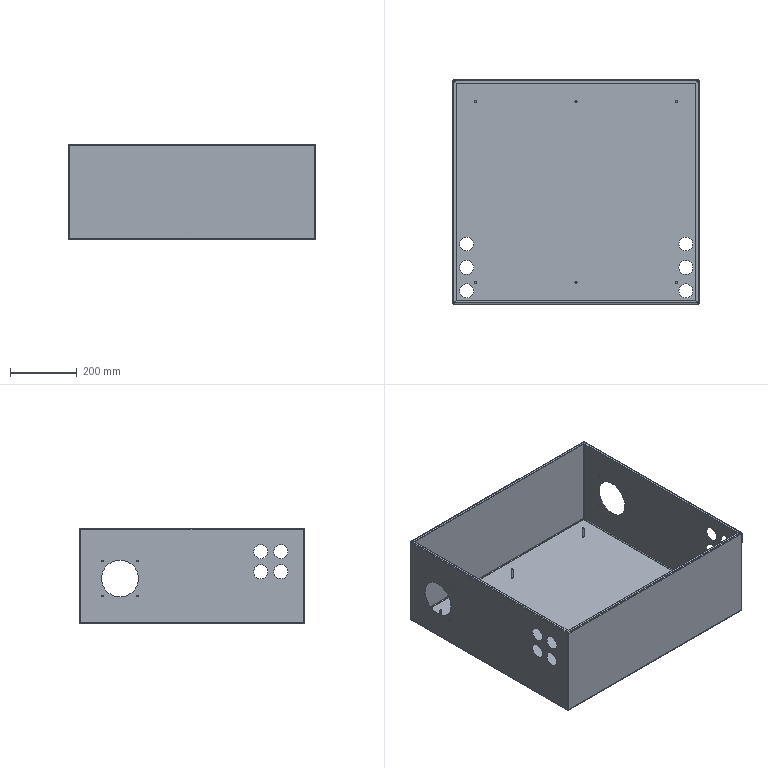Part | SolidWorks | features ICE 4, EdgeFlange 2, FlatPattern 1, LPattern 1, SMBaseFlange 1, SheetMetal 1 | 1 solid | 136 faces | box 736 x 670 x 285 mm | volume 1900443 mm3 | cylinder 76 | plane 44 | spline 16 | commonest cylinder face diameters 42 x28 5 x16 6 x12 4 x8 7 x8 110 x4